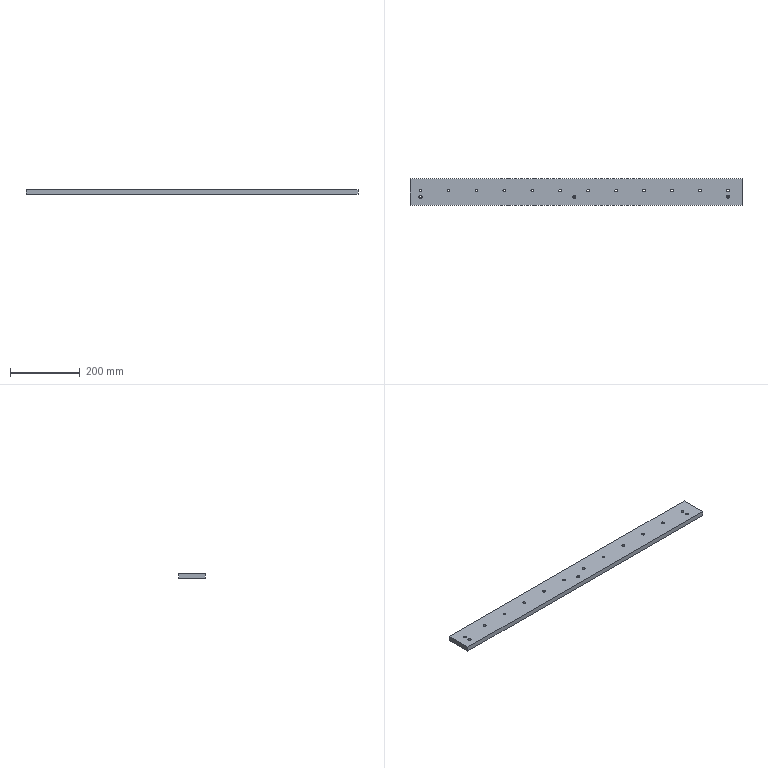Part | STEP file | [07] | 1 solid | 51 faces | box 950 x 75 x 14 mm | volume 987198 mm3 | cylinder 36 | plane 9 | cone 6 | commonest cylinder face diameters 8 x30 6 x6